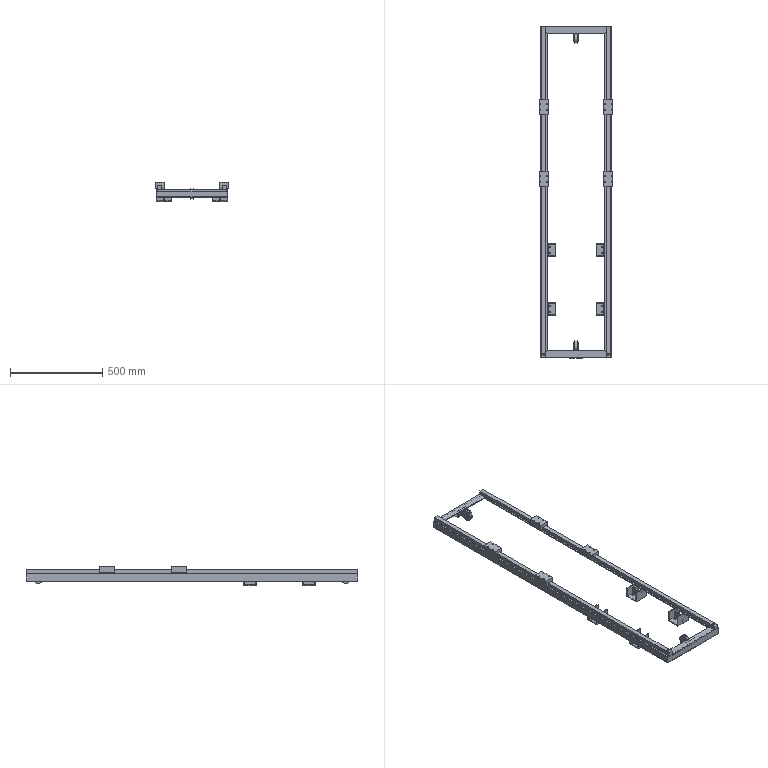Part | SolidWorks | 18 solids | 464 faces | box 398 x 1800 x 104 mm | volume 4027094 mm3 | cylinder 238 | plane 194 | cone 32 | commonest cylinder face diameters 6.5 x152 5 x48 2.667 x8 60 x8 35 x6 7 x4